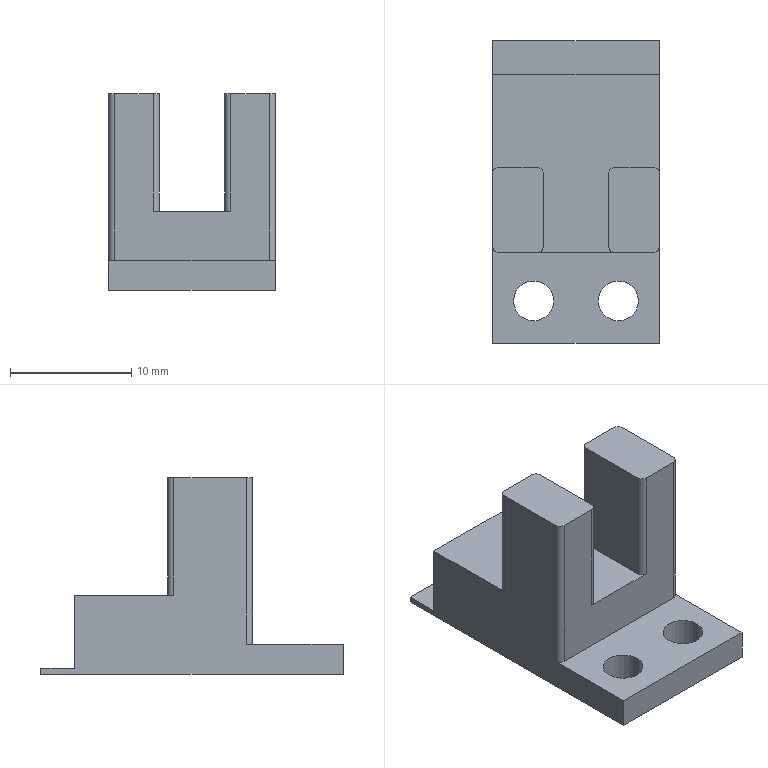Part | NX | features BREP 1 | 1 solid | 28 faces | box 13.8 x 25 x 16.25 mm | volume 2130 mm3 | plane 16 | cylinder 12 | commonest cylinder face diameters 1 x8 3.3 x4
STEP:
#1=CARTESIAN_POINT('',(-3.2,7.5,16.25));
#2=VERTEX_POINT('',#1);
#3=CARTESIAN_POINT('',(-2.7,8.,16.25));
#4=VERTEX_POINT('',#3);
#5=CARTESIAN_POINT('',(-3.2,8.,16.25));
#6=DIRECTION('',(0.,0.,1.));
#7=DIRECTION('',(-1.,0.,0.));
#8=AXIS2_PLACEMENT_3D('',#5,#6,#7);
#9=CIRCLE('',#8,0.5);
#10=EDGE_CURVE('',#2,#4,#9,.T.);
#11=ORIENTED_EDGE('',*,*,#10,.F.);
#12=CARTESIAN_POINT('',(-3.2,7.5,6.55));
#13=VERTEX_POINT('',#12);
#14=CARTESIAN_POINT('',(-3.2,7.5,6.55));
#15=DIRECTION('',(0.,0.,1.));
#16=VECTOR('',#15,1000.);
#17=LINE('',#14,#16);
#18=EDGE_CURVE('',#13,#2,#17,.T.);
#19=ORIENTED_EDGE('',*,*,#18,.F.);
#20=CARTESIAN_POINT('',(-2.7,8.,6.55));
#21=VERTEX_POINT('',#20);
#22=CARTESIAN_POINT('',(-3.2,8.,6.55));
#23=DIRECTION('',(0.,0.,-1.));
#24=DIRECTION('',(-1.,0.,0.));
#25=AXIS2_PLACEMENT_3D('',#22,#23,#24);
#26=CIRCLE('',#25,0.5);
#27=EDGE_CURVE('',#21,#13,#26,.T.);
#28=ORIENTED_EDGE('',*,*,#27,.F.);
#29=CARTESIAN_POINT('',(-2.7,8.,16.25));
#30=DIRECTION('',(0.,0.,-1.));
#31=VECTOR('',#30,1000.);
#32=LINE('',#29,#31);
#33=EDGE_CURVE('',#4,#21,#32,.T.);
#34=ORIENTED_EDGE('',*,*,#33,.F.);
#35=EDGE_LOOP('',(#11,#19,#28,#34));
#36=FACE_BOUND('',#35,.T.);
#37=CARTESIAN_POINT('',(-3.2,8.,16.25));
#38=DIRECTION('',(0.,0.,-1.));
#39=DIRECTION('',(-1.,0.,0.));
#40=AXIS2_PLACEMENT_3D('',#37,#38,#39);
#41=CYLINDRICAL_SURFACE('',#40,0.5);
#42=ADVANCED_FACE('',(#36),#41,.T.);
#43=CARTESIAN_POINT('',(2.7,8.,16.25));
#44=VERTEX_POINT('',#43);
#45=CARTESIAN_POINT('',(3.2,7.5,16.25));
#46=VERTEX_POINT('',#45);
#47=CARTESIAN_POINT('',(3.2,8.,16.25));
#48=DIRECTION('',(0.,0.,1.));
#49=DIRECTION('',(1.,0.,0.));
#50=AXIS2_PLACEMENT_3D('',#47,#48,#49);
#51=CIRCLE('',#50,0.5);
#52=EDGE_CURVE('',#44,#46,#51,.T.);
#53=ORIENTED_EDGE('',*,*,#52,.F.);
#54=CARTESIAN_POINT('',(2.7,8.,6.55));
#55=VERTEX_POINT('',#54);
#56=CARTESIAN_POINT('',(2.7,8.,16.25));
#57=DIRECTION('',(0.,0.,1.));
#58=VECTOR('',#57,1000.);
#59=LINE('',#56,#58);
#60=EDGE_CURVE('',#55,#44,#59,.T.);
#61=ORIENTED_EDGE('',*,*,#60,.F.);
#62=CARTESIAN_POINT('',(3.2,7.5,6.55));
#63=VERTEX_POINT('',#62);
#64=CARTESIAN_POINT('',(3.2,8.,6.55));
#65=DIRECTION('',(0.,0.,-1.));
#66=DIRECTION('',(-1.,0.,0.));
#67=AXIS2_PLACEMENT_3D('',#64,#65,#66);
#68=CIRCLE('',#67,0.5);
#69=EDGE_CURVE('',#63,#55,#68,.T.);
#70=ORIENTED_EDGE('',*,*,#69,.F.);
#71=CARTESIAN_POINT('',(3.2,7.5,6.55));
#72=DIRECTION('',(0.,0.,-1.));
#73=VECTOR('',#72,1000.);
#74=LINE('',#71,#73);
#75=EDGE_CURVE('',#46,#63,#74,.T.);
#76=ORIENTED_EDGE('',*,*,#75,.F.);
#77=EDGE_LOOP('',(#53,#61,#70,#76));
#78=FACE_BOUND('',#77,.T.);
#79=CARTESIAN_POINT('',(3.2,8.,6.55));
#80=DIRECTION('',(0.,0.,-1.));
#81=DIRECTION('',(-1.,0.,0.));
#82=AXIS2_PLACEMENT_3D('',#79,#80,#81);
#83=CYLINDRICAL_SURFACE('',#82,0.5);
#84=ADVANCED_FACE('',(#78),#83,.T.);
#85=CARTESIAN_POINT('',(3.2,14.5,16.25));
#86=VERTEX_POINT('',#85);
#87=CARTESIAN_POINT('',(2.7,14.,16.25));
#88=VERTEX_POINT('',#87);
#89=CARTESIAN_POINT('',(3.2,14.,16.25));
#90=DIRECTION('',(0.,0.,1.));
#91=DIRECTION('',(1.,0.,0.));
#92=AXIS2_PLACEMENT_3D('',#89,#90,#91);
#93=CIRCLE('',#92,0.5);
#94=EDGE_CURVE('',#86,#88,#93,.T.);
#95=ORIENTED_EDGE('',*,*,#94,.F.);
#96=CARTESIAN_POINT('',(3.2,14.5,6.55));
#97=VERTEX_POINT('',#96);
#98=CARTESIAN_POINT('',(3.2,14.5,16.25));
#99=DIRECTION('',(0.,0.,1.));
#100=VECTOR('',#99,1000.);
#101=LINE('',#98,#100);
#102=EDGE_CURVE('',#97,#86,#101,.T.);
#103=ORIENTED_EDGE('',*,*,#102,.F.);
#104=CARTESIAN_POINT('',(2.7,14.,6.55));
#105=VERTEX_POINT('',#104);
#106=CARTESIAN_POINT('',(3.2,14.,6.55));
#107=DIRECTION('',(0.,0.,-1.));
#108=DIRECTION('',(-1.,0.,0.));
#109=AXIS2_PLACEMENT_3D('',#106,#107,#108);
#110=CIRCLE('',#109,0.5);
#111=EDGE_CURVE('',#105,#97,#110,.T.);
#112=ORIENTED_EDGE('',*,*,#111,.F.);
#113=CARTESIAN_POINT('',(2.7,14.,16.25));
#114=DIRECTION('',(0.,0.,-1.));
#115=VECTOR('',#114,1000.);
#116=LINE('',#113,#115);
#117=EDGE_CURVE('',#88,#105,#116,.T.);
#118=ORIENTED_EDGE('',*,*,#117,.F.);
#119=EDGE_LOOP('',(#95,#103,#112,#118));
#120=FACE_BOUND('',#119,.T.);
#121=CARTESIAN_POINT('',(3.2,14.,16.25));
#122=DIRECTION('',(0.,0.,-1.));
#123=DIRECTION('',(-1.,0.,0.));
#124=AXIS2_PLACEMENT_3D('',#121,#122,#123);
#125=CYLINDRICAL_SURFACE('',#124,0.5);
#126=ADVANCED_FACE('',(#120),#125,.T.);
#127=CARTESIAN_POINT('',(-2.7,14.,16.25));
#128=VERTEX_POINT('',#127);
#129=CARTESIAN_POINT('',(-3.2,14.5,16.25));
#130=VERTEX_POINT('',#129);
#131=CARTESIAN_POINT('',(-3.2,14.,16.25));
#132=DIRECTION('',(0.,0.,1.));
#133=DIRECTION('',(-1.,0.,0.));
#134=AXIS2_PLACEMENT_3D('',#131,#132,#133);
#135=CIRCLE('',#134,0.5);
#136=EDGE_CURVE('',#128,#130,#135,.T.);
#137=ORIENTED_EDGE('',*,*,#136,.F.);
#138=CARTESIAN_POINT('',(-2.7,14.,6.55));
#139=VERTEX_POINT('',#138);
#140=CARTESIAN_POINT('',(-2.7,14.,16.25));
#141=DIRECTION('',(0.,0.,1.));
#142=VECTOR('',#141,1000.);
#143=LINE('',#140,#142);
#144=EDGE_CURVE('',#139,#128,#143,.T.);
#145=ORIENTED_EDGE('',*,*,#144,.F.);
#146=CARTESIAN_POINT('',(-3.2,14.5,6.55));
#147=VERTEX_POINT('',#146);
#148=CARTESIAN_POINT('',(-3.2,14.,6.55));
#149=DIRECTION('',(0.,0.,-1.));
#150=DIRECTION('',(-1.,0.,0.));
#151=AXIS2_PLACEMENT_3D('',#148,#149,#150);
#152=CIRCLE('',#151,0.5);
#153=EDGE_CURVE('',#147,#139,#152,.T.);
#154=ORIENTED_EDGE('',*,*,#153,.F.);
#155=CARTESIAN_POINT('',(-3.2,14.5,16.25));
#156=DIRECTION('',(0.,0.,-1.));
#157=VECTOR('',#156,1000.);
#158=LINE('',#155,#157);
#159=EDGE_CURVE('',#130,#147,#158,.T.);
#160=ORIENTED_EDGE('',*,*,#159,.F.);
#161=EDGE_LOOP('',(#137,#145,#154,#160));
#162=FACE_BOUND('',#161,.T.);
#163=CARTESIAN_POINT('',(-3.2,14.,16.25));
#164=DIRECTION('',(0.,0.,-1.));
#165=DIRECTION('',(-1.,0.,0.));
#166=AXIS2_PLACEMENT_3D('',#163,#164,#165);
#167=CYLINDRICAL_SURFACE('',#166,0.5);
#168=ADVANCED_FACE('',(#162),#167,.T.);
#169=CARTESIAN_POINT('',(-6.4,14.5,16.25));
#170=VERTEX_POINT('',#169);
#171=CARTESIAN_POINT('',(-6.9,14.,16.25));
#172=VERTEX_POINT('',#171);
#173=CARTESIAN_POINT('',(-6.4,14.,16.25));
#174=DIRECTION('',(0.,0.,1.));
#175=DIRECTION('',(-1.,0.,0.));
#176=AXIS2_PLACEMENT_3D('',#173,#174,#175);
#177=CIRCLE('',#176,0.5);
#178=EDGE_CURVE('',#170,#172,#177,.T.);
#179=ORIENTED_EDGE('',*,*,#178,.F.);
#180=CARTESIAN_POINT('',(-6.4,14.5,6.55));
#181=VERTEX_POINT('',#180);
#182=CARTESIAN_POINT('',(-6.4,14.5,16.25));
#183=DIRECTION('',(0.,0.,1.));
#184=VECTOR('',#183,1000.);
#185=LINE('',#182,#184);
#186=EDGE_CURVE('',#181,#170,#185,.T.);
#187=ORIENTED_EDGE('',*,*,#186,.F.);
#188=CARTESIAN_POINT('',(-6.9,14.,6.55));
#189=VERTEX_POINT('',#188);
#190=CARTESIAN_POINT('',(-6.4,14.,6.55));
#191=DIRECTION('',(0.,0.,-1.));
#192=DIRECTION('',(-1.,0.,0.));
#193=AXIS2_PLACEMENT_3D('',#190,#191,#192);
#194=CIRCLE('',#193,0.5);
#195=EDGE_CURVE('',#189,#181,#194,.T.);
#196=ORIENTED_EDGE('',*,*,#195,.F.);
#197=CARTESIAN_POINT('',(-6.9,14.,2.5));
#198=DIRECTION('',(0.,0.,-1.));
#199=VECTOR('',#198,1000.);
#200=LINE('',#197,#199);
#201=EDGE_CURVE('',#172,#189,#200,.T.);
#202=ORIENTED_EDGE('',*,*,#201,.F.);
#203=EDGE_LOOP('',(#179,#187,#196,#202));
#204=FACE_BOUND('',#203,.T.);
#205=CARTESIAN_POINT('',(-6.4,14.,2.5));
#206=DIRECTION('',(0.,0.,-1.));
#207=DIRECTION('',(-1.,0.,0.));
#208=AXIS2_PLACEMENT_3D('',#205,#206,#207);
#209=CYLINDRICAL_SURFACE('',#208,0.5);
#210=ADVANCED_FACE('',(#204),#209,.T.);
#211=CARTESIAN_POINT('',(-6.9,8.,16.25));
#212=VERTEX_POINT('',#211);
#213=CARTESIAN_POINT('',(-6.4,7.5,16.25));
#214=VERTEX_POINT('',#213);
#215=CARTESIAN_POINT('',(-6.4,8.,16.25));
#216=DIRECTION('',(0.,0.,1.));
#217=DIRECTION('',(-1.,0.,0.));
#218=AXIS2_PLACEMENT_3D('',#215,#216,#217);
#219=CIRCLE('',#218,0.5);
#220=EDGE_CURVE('',#212,#214,#219,.T.);
#221=ORIENTED_EDGE('',*,*,#220,.F.);
#222=CARTESIAN_POINT('',(-6.9,8.,2.5));
#223=VERTEX_POINT('',#222);
#224=CARTESIAN_POINT('',(-6.9,8.,2.5));
#225=DIRECTION('',(0.,0.,1.));
#226=VECTOR('',#225,1000.);
#227=LINE('',#224,#226);
#228=EDGE_CURVE('',#223,#212,#227,.T.);
#229=ORIENTED_EDGE('',*,*,#228,.F.);
#230=CARTESIAN_POINT('',(-6.4,7.5,2.5));
#231=VERTEX_POINT('',#230);
#232=CARTESIAN_POINT('',(-6.4,8.,2.5));
#233=DIRECTION('',(0.,0.,-1.));
#234=DIRECTION('',(1.,0.,0.));
#235=AXIS2_PLACEMENT_3D('',#232,#233,#234);
#236=CIRCLE('',#235,0.5);
#237=EDGE_CURVE('',#231,#223,#236,.T.);
#238=ORIENTED_EDGE('',*,*,#237,.F.);
#239=CARTESIAN_POINT('',(-6.4,7.5,6.55));
#240=DIRECTION('',(0.,0.,-1.));
#241=VECTOR('',#240,1000.);
#242=LINE('',#239,#241);
#243=EDGE_CURVE('',#214,#231,#242,.T.);
#244=ORIENTED_EDGE('',*,*,#243,.F.);
#245=EDGE_LOOP('',(#221,#229,#238,#244));
#246=FACE_BOUND('',#245,.T.);
#247=CARTESIAN_POINT('',(-6.4,8.,6.55));
#248=DIRECTION('',(0.,0.,-1.));
#249=DIRECTION('',(-1.,0.,0.));
#250=AXIS2_PLACEMENT_3D('',#247,#248,#249);
#251=CYLINDRICAL_SURFACE('',#250,0.5);
#252=ADVANCED_FACE('',(#246),#251,.T.);
#253=CARTESIAN_POINT('',(6.4,7.5,16.25));
#254=VERTEX_POINT('',#253);
#255=CARTESIAN_POINT('',(6.9,8.,16.25));
#256=VERTEX_POINT('',#255);
#257=CARTESIAN_POINT('',(6.4,8.,16.25));
#258=DIRECTION('',(0.,0.,1.));
#259=DIRECTION('',(1.,0.,0.));
#260=AXIS2_PLACEMENT_3D('',#257,#258,#259);
#261=CIRCLE('',#260,0.5);
#262=EDGE_CURVE('',#254,#256,#261,.T.);
#263=ORIENTED_EDGE('',*,*,#262,.F.);
#264=CARTESIAN_POINT('',(6.4,7.5,2.5));
#265=VERTEX_POINT('',#264);
#266=CARTESIAN_POINT('',(6.4,7.5,6.55));
#267=DIRECTION('',(0.,0.,1.));
#268=VECTOR('',#267,1000.);
#269=LINE('',#266,#268);
#270=EDGE_CURVE('',#265,#254,#269,.T.);
#271=ORIENTED_EDGE('',*,*,#270,.F.);
#272=CARTESIAN_POINT('',(6.9,8.,2.5));
#273=VERTEX_POINT('',#272);
#274=CARTESIAN_POINT('',(6.4,8.,2.5));
#275=DIRECTION('',(0.,0.,-1.));
#276=DIRECTION('',(1.,0.,0.));
#277=AXIS2_PLACEMENT_3D('',#274,#275,#276);
#278=CIRCLE('',#277,0.5);
#279=EDGE_CURVE('',#273,#265,#278,.T.);
#280=ORIENTED_EDGE('',*,*,#279,.F.);
#281=CARTESIAN_POINT('',(6.9,8.,2.5));
#282=DIRECTION('',(0.,0.,-1.));
#283=VECTOR('',#282,1000.);
#284=LINE('',#281,#283);
#285=EDGE_CURVE('',#256,#273,#284,.T.);
#286=ORIENTED_EDGE('',*,*,#285,.F.);
#287=EDGE_LOOP('',(#263,#271,#280,#286));
#288=FACE_BOUND('',#287,.T.);
#289=CARTESIAN_POINT('',(6.4,8.,2.5));
#290=DIRECTION('',(0.,0.,-1.));
#291=DIRECTION('',(-1.,0.,0.));
#292=AXIS2_PLACEMENT_3D('',#289,#290,#291);
#293=CYLINDRICAL_SURFACE('',#292,0.5);
#294=ADVANCED_FACE('',(#288),#293,.T.);
#295=CARTESIAN_POINT('',(6.9,14.,16.25));
#296=VERTEX_POINT('',#295);
#297=CARTESIAN_POINT('',(6.4,14.5,16.25));
#298=VERTEX_POINT('',#297);
#299=CARTESIAN_POINT('',(6.4,14.,16.25));
#300=DIRECTION('',(0.,0.,1.));
#301=DIRECTION('',(1.,0.,0.));
#302=AXIS2_PLACEMENT_3D('',#299,#300,#301);
#303=CIRCLE('',#302,0.5);
#304=EDGE_CURVE('',#296,#298,#303,.T.);
#305=ORIENTED_EDGE('',*,*,#304,.F.);
#306=CARTESIAN_POINT('',(6.9,14.,6.55));
#307=VERTEX_POINT('',#306);
#308=CARTESIAN_POINT('',(6.9,14.,2.5));
#309=DIRECTION('',(0.,0.,1.));
#310=VECTOR('',#309,1000.);
#311=LINE('',#308,#310);
#312=EDGE_CURVE('',#307,#296,#311,.T.);
#313=ORIENTED_EDGE('',*,*,#312,.F.);
#314=CARTESIAN_POINT('',(6.4,14.5,6.55));
#315=VERTEX_POINT('',#314);
#316=CARTESIAN_POINT('',(6.4,14.,6.55));
#317=DIRECTION('',(0.,0.,-1.));
#318=DIRECTION('',(-1.,0.,0.));
#319=AXIS2_PLACEMENT_3D('',#316,#317,#318);
#320=CIRCLE('',#319,0.5);
#321=EDGE_CURVE('',#315,#307,#320,.T.);
#322=ORIENTED_EDGE('',*,*,#321,.F.);
#323=CARTESIAN_POINT('',(6.4,14.5,16.25));
#324=DIRECTION('',(0.,0.,-1.));
#325=VECTOR('',#324,1000.);
#326=LINE('',#323,#325);
#327=EDGE_CURVE('',#298,#315,#326,.T.);
#328=ORIENTED_EDGE('',*,*,#327,.F.);
#329=EDGE_LOOP('',(#305,#313,#322,#328));
#330=FACE_BOUND('',#329,.T.);
#331=CARTESIAN_POINT('',(6.4,14.,16.25));
#332=DIRECTION('',(0.,0.,-1.));
#333=DIRECTION('',(-1.,0.,0.));
#334=AXIS2_PLACEMENT_3D('',#331,#332,#333);
#335=CYLINDRICAL_SURFACE('',#334,0.5);
#336=ADVANCED_FACE('',(#330),#335,.T.);
#337=CARTESIAN_POINT('',(-6.9,25.,0.5));
#338=VERTEX_POINT('',#337);
#339=CARTESIAN_POINT('',(-6.9,22.2,0.5));
#340=VERTEX_POINT('',#339);
#341=CARTESIAN_POINT('',(-6.9,22.2,0.5));
#342=DIRECTION('',(0.,-1.,0.));
#343=VECTOR('',#342,1000.);
#344=LINE('',#341,#343);
#345=EDGE_CURVE('',#338,#340,#344,.T.);
#346=ORIENTED_EDGE('',*,*,#345,.T.);
#347=CARTESIAN_POINT('',(6.9,22.2,0.5));
#348=VERTEX_POINT('',#347);
#349=CARTESIAN_POINT('',(-6.9,22.2,0.5));
#350=DIRECTION('',(1.,0.,0.));
#351=VECTOR('',#350,1000.);
#352=LINE('',#349,#351);
#353=EDGE_CURVE('',#340,#348,#352,.T.);
#354=ORIENTED_EDGE('',*,*,#353,.T.);
#355=CARTESIAN_POINT('',(6.9,25.,0.5));
#356=VERTEX_POINT('',#355);
#357=CARTESIAN_POINT('',(6.9,22.2,0.5));
#358=DIRECTION('',(0.,1.,0.));
#359=VECTOR('',#358,1000.);
#360=LINE('',#357,#359);
#361=EDGE_CURVE('',#348,#356,#360,.T.);
#362=ORIENTED_EDGE('',*,*,#361,.T.);
#363=CARTESIAN_POINT('',(-6.9,25.,0.5));
#364=DIRECTION('',(-1.,0.,0.));
#365=VECTOR('',#364,1000.);
#366=LINE('',#363,#365);
#367=EDGE_CURVE('',#356,#338,#366,.T.);
#368=ORIENTED_EDGE('',*,*,#367,.T.);
#369=EDGE_LOOP('',(#346,#354,#362,#368));
#370=FACE_BOUND('',#369,.T.);
#371=CARTESIAN_POINT('',(-6.9,25.,0.5));
#372=DIRECTION('',(0.,0.,-1.));
#373=DIRECTION('',(-1.,0.,0.));
#374=AXIS2_PLACEMENT_3D('',#371,#372,#373);
#375=PLANE('',#374);
#376=ADVANCED_FACE('',(#370),#375,.F.);
#377=CARTESIAN_POINT('',(1.85,3.5,2.5));
#378=VERTEX_POINT('',#377);
#379=CARTESIAN_POINT('',(1.85,3.5,0.));
#380=VERTEX_POINT('',#379);
#381=CARTESIAN_POINT('',(1.85,3.5,-7.2));
#382=DIRECTION('',(0.,0.,1.));
#383=VECTOR('',#382,1000.);
#384=LINE('',#381,#383);
#385=EDGE_CURVE('',#378,#380,#384,.F.);
#386=ORIENTED_EDGE('',*,*,#385,.T.);
#387=CARTESIAN_POINT('',(5.15,3.5,0.));
#388=VERTEX_POINT('',#387);
#389=CARTESIAN_POINT('',(3.5,3.5,0.));
#390=DIRECTION('',(0.,0.,1.));
#391=DIRECTION('',(1.,0.,0.));
#392=AXIS2_PLACEMENT_3D('',#389,#390,#391);
#393=CIRCLE('',#392,1.65);
#394=EDGE_CURVE('',#388,#380,#393,.T.);
#395=ORIENTED_EDGE('',*,*,#394,.F.);
#396=CARTESIAN_POINT('',(5.15,3.5,2.5));
#397=VERTEX_POINT('',#396);
#398=CARTESIAN_POINT('',(5.15,3.5,-7.2));
#399=DIRECTION('',(0.,0.,1.));
#400=VECTOR('',#399,1000.);
#401=LINE('',#398,#400);
#402=EDGE_CURVE('',#397,#388,#401,.F.);
#403=ORIENTED_EDGE('',*,*,#402,.F.);
#404=CARTESIAN_POINT('',(3.5,3.5,2.5));
#405=DIRECTION('',(0.,0.,1.));
#406=DIRECTION('',(1.,0.,0.));
#407=AXIS2_PLACEMENT_3D('',#404,#405,#406);
#408=CIRCLE('',#407,1.65);
#409=EDGE_CURVE('',#397,#378,#408,.T.);
#410=ORIENTED_EDGE('',*,*,#409,.T.);
#411=EDGE_LOOP('',(#386,#395,#403,#410));
#412=FACE_BOUND('',#411,.T.);
#413=CARTESIAN_POINT('',(3.5,3.5,-7.2));
#414=DIRECTION('',(0.,0.,1.));
#415=DIRECTION('',(1.,0.,0.));
#416=AXIS2_PLACEMENT_3D('',#413,#414,#415);
#417=CYLINDRICAL_SURFACE('',#416,1.65);
#418=ADVANCED_FACE('',(#412),#417,.F.);
#419=CARTESIAN_POINT('',(-5.15,3.5,2.5));
#420=VERTEX_POINT('',#419);
#421=CARTESIAN_POINT('',(-5.15,3.5,0.));
#422=VERTEX_POINT('',#421);
#423=CARTESIAN_POINT('',(-5.15,3.5,-7.2));
#424=DIRECTION('',(0.,0.,1.));
#425=VECTOR('',#424,1000.);
#426=LINE('',#423,#425);
#427=EDGE_CURVE('',#420,#422,#426,.F.);
#428=ORIENTED_EDGE('',*,*,#427,.T.);
#429=CARTESIAN_POINT('',(-1.85,3.5,0.));
#430=VERTEX_POINT('',#429);
#431=CARTESIAN_POINT('',(-3.5,3.5,0.));
#432=DIRECTION('',(0.,0.,1.));
#433=DIRECTION('',(1.,0.,0.));
#434=AXIS2_PLACEMENT_3D('',#431,#432,#433);
#435=CIRCLE('',#434,1.65);
#436=EDGE_CURVE('',#430,#422,#435,.T.);
#437=ORIENTED_EDGE('',*,*,#436,.F.);
#438=CARTESIAN_POINT('',(-1.85,3.5,2.5));
#439=VERTEX_POINT('',#438);
#440=CARTESIAN_POINT('',(-1.85,3.5,-7.2));
#441=DIRECTION('',(0.,0.,1.));
#442=VECTOR('',#441,1000.);
#443=LINE('',#440,#442);
#444=EDGE_CURVE('',#439,#430,#443,.F.);
#445=ORIENTED_EDGE('',*,*,#444,.F.);
#446=CARTESIAN_POINT('',(-3.5,3.5,2.5));
#447=DIRECTION('',(0.,0.,1.));
#448=DIRECTION('',(1.,0.,0.));
#449=AXIS2_PLACEMENT_3D('',#446,#447,#448);
#450=CIRCLE('',#449,1.65);
#451=EDGE_CURVE('',#439,#420,#450,.T.);
#452=ORIENTED_EDGE('',*,*,#451,.T.);
#453=EDGE_LOOP('',(#428,#437,#445,#452));
#454=FACE_BOUND('',#453,.T.);
#455=CARTESIAN_POINT('',(-3.5,3.5,-7.2));
#456=DIRECTION('',(0.,0.,1.));
#457=DIRECTION('',(1.,0.,0.));
#458=AXIS2_PLACEMENT_3D('',#455,#456,#457);
#459=CYLINDRICAL_SURFACE('',#458,1.65);
#460=ADVANCED_FACE('',(#454),#459,.F.);
#461=CARTESIAN_POINT('',(6.9,7.5,16.25));
#462=DIRECTION('',(0.,1.,0.));
#463=VECTOR('',#462,1000.);
#464=LINE('',#461,#463);
#465=EDGE_CURVE('',#256,#296,#464,.T.);
#466=ORIENTED_EDGE('',*,*,#465,.T.);
#467=ORIENTED_EDGE('',*,*,#304,.T.);
#468=CARTESIAN_POINT('',(6.9,14.5,16.25));
#469=DIRECTION('',(-1.,0.,0.));
#470=VECTOR('',#469,1000.);
#471=LINE('',#468,#470);
#472=EDGE_CURVE('',#298,#86,#471,.T.);
#473=ORIENTED_EDGE('',*,*,#472,.T.);
#474=ORIENTED_EDGE('',*,*,#94,.T.);
#475=CARTESIAN_POINT('',(2.7,7.5,16.25));
#476=DIRECTION('',(0.,-1.,0.));
#477=VECTOR('',#476,1000.);
#478=LINE('',#475,#477);
#479=EDGE_CURVE('',#88,#44,#478,.T.);
#480=ORIENTED_EDGE('',*,*,#479,.T.);
#481=ORIENTED_EDGE('',*,*,#52,.T.);
#482=CARTESIAN_POINT('',(6.9,7.5,16.25));
#483=DIRECTION('',(1.,0.,0.));
#484=VECTOR('',#483,1000.);
#485=LINE('',#482,#484);
#486=EDGE_CURVE('',#46,#254,#485,.T.);
#487=ORIENTED_EDGE('',*,*,#486,.T.);
#488=ORIENTED_EDGE('',*,*,#262,.T.);
#489=EDGE_LOOP('',(#466,#467,#473,#474,#480,#481,#487,#488));
#490=FACE_BOUND('',#489,.T.);
#491=CARTESIAN_POINT('',(6.9,14.5,16.25));
#492=DIRECTION('',(0.,0.,1.));
#493=DIRECTION('',(1.,0.,0.));
#494=AXIS2_PLACEMENT_3D('',#491,#492,#493);
#495=PLANE('',#494);
#496=ADVANCED_FACE('',(#490),#495,.T.);
#497=ORIENTED_EDGE('',*,*,#479,.F.);
#498=ORIENTED_EDGE('',*,*,#117,.T.);
#499=CARTESIAN_POINT('',(2.7,7.5,6.55));
#500=DIRECTION('',(0.,-1.,0.));
#501=VECTOR('',#500,1000.);
#502=LINE('',#499,#501);
#503=EDGE_CURVE('',#105,#55,#502,.T.);
#504=ORIENTED_EDGE('',*,*,#503,.T.);
#505=ORIENTED_EDGE('',*,*,#60,.T.);
#506=EDGE_LOOP('',(#497,#498,#504,#505));
#507=FACE_BOUND('',#506,.T.);
#508=CARTESIAN_POINT('',(2.7,7.5,16.25));
#509=DIRECTION('',(1.,0.,0.));
#510=DIRECTION('',(0.,0.,-1.));
#511=AXIS2_PLACEMENT_3D('',#508,#509,#510);
#512=PLANE('',#511);
#513=ADVANCED_FACE('',(#507),#512,.F.);
#514=ORIENTED_EDGE('',*,*,#472,.F.);
#515=ORIENTED_EDGE('',*,*,#327,.T.);
#516=CARTESIAN_POINT('',(6.9,14.5,6.55));
#517=DIRECTION('',(-1.,0.,0.));
#518=VECTOR('',#517,1000.);
#519=LINE('',#516,#518);
#520=EDGE_CURVE('',#315,#97,#519,.T.);
#521=ORIENTED_EDGE('',*,*,#520,.T.);
#522=ORIENTED_EDGE('',*,*,#102,.T.);
#523=EDGE_LOOP('',(#514,#515,#521,#522));
#524=FACE_BOUND('',#523,.T.);
#525=CARTESIAN_POINT('',(6.9,14.5,16.25));
#526=DIRECTION('',(0.,-1.,0.));
#527=DIRECTION('',(0.,0.,-1.));
#528=AXIS2_PLACEMENT_3D('',#525,#526,#527);
#529=PLANE('',#528);
#530=ADVANCED_FACE('',(#524),#529,.F.);
#531=CARTESIAN_POINT('',(-6.9,7.5,16.25));
#532=DIRECTION('',(0.,-1.,0.));
#533=VECTOR('',#532,1000.);
#534=LINE('',#531,#533);
#535=EDGE_CURVE('',#172,#212,#534,.T.);
#536=ORIENTED_EDGE('',*,*,#535,.T.);
#537=ORIENTED_EDGE('',*,*,#220,.T.);
#538=CARTESIAN_POINT('',(-6.9,7.5,16.25));
#539=DIRECTION('',(1.,0.,0.));
#540=VECTOR('',#539,1000.);
#541=LINE('',#538,#540);
#542=EDGE_CURVE('',#214,#2,#541,.T.);
#543=ORIENTED_EDGE('',*,*,#542,.T.);
#544=ORIENTED_EDGE('',*,*,#10,.T.);
#545=CARTESIAN_POINT('',(-2.7,7.5,16.25));
#546=DIRECTION('',(0.,1.,0.));
#547=VECTOR('',#546,1000.);
#548=LINE('',#545,#547);
#549=EDGE_CURVE('',#4,#128,#548,.T.);
#550=ORIENTED_EDGE('',*,*,#549,.T.);
#551=ORIENTED_EDGE('',*,*,#136,.T.);
#552=CARTESIAN_POINT('',(-6.9,14.5,16.25));
#553=DIRECTION('',(-1.,0.,0.));
#554=VECTOR('',#553,1000.);
#555=LINE('',#552,#554);
#556=EDGE_CURVE('',#130,#170,#555,.T.);
#557=ORIENTED_EDGE('',*,*,#556,.T.);
#558=ORIENTED_EDGE('',*,*,#178,.T.);
#559=EDGE_LOOP('',(#536,#537,#543,#544,#550,#551,#557,#558));
#560=FACE_BOUND('',#559,.T.);
#561=CARTESIAN_POINT('',(-6.9,14.5,16.25));
#562=DIRECTION('',(0.,0.,-1.));
#563=DIRECTION('',(-1.,0.,0.));
#564=AXIS2_PLACEMENT_3D('',#561,#562,#563);
#565=PLANE('',#564);
#566=ADVANCED_FACE('',(#560),#565,.F.);
#567=CARTESIAN_POINT('',(-6.9,14.5,6.55));
#568=DIRECTION('',(-1.,0.,0.));
#569=VECTOR('',#568,1000.);
#570=LINE('',#567,#569);
#571=EDGE_CURVE('',#147,#181,#570,.T.);
#572=ORIENTED_EDGE('',*,*,#571,.T.);
#573=ORIENTED_EDGE('',*,*,#186,.T.);
#574=ORIENTED_EDGE('',*,*,#556,.F.);
#575=ORIENTED_EDGE('',*,*,#159,.T.);
#576=EDGE_LOOP('',(#572,#573,#574,#575));
#577=FACE_BOUND('',#576,.T.);
#578=CARTESIAN_POINT('',(-6.9,14.5,16.25));
#579=DIRECTION('',(0.,-1.,0.));
#580=DIRECTION('',(0.,0.,-1.));
#581=AXIS2_PLACEMENT_3D('',#578,#579,#580);
#582=PLANE('',#581);
#583=ADVANCED_FACE('',(#577),#582,.F.);
#584=CARTESIAN_POINT('',(-2.7,7.5,6.55));
#585=DIRECTION('',(0.,1.,0.));
#586=VECTOR('',#585,1000.);
#587=LINE('',#584,#586);
#588=EDGE_CURVE('',#21,#139,#587,.T.);
#589=ORIENTED_EDGE('',*,*,#588,.T.);
#590=ORIENTED_EDGE('',*,*,#144,.T.);
#591=ORIENTED_EDGE('',*,*,#549,.F.);
#592=ORIENTED_EDGE('',*,*,#33,.T.);
#593=EDGE_LOOP('',(#589,#590,#591,#592));
#594=FACE_BOUND('',#593,.T.);
#595=CARTESIAN_POINT('',(-2.7,7.5,16.25));
#596=DIRECTION('',(-1.,0.,0.));
#597=DIRECTION('',(0.,0.,1.));
#598=AXIS2_PLACEMENT_3D('',#595,#596,#597);
#599=PLANE('',#598);
#600=ADVANCED_FACE('',(#594),#599,.F.);
#601=CARTESIAN_POINT('',(6.9,22.2,6.55));
#602=VERTEX_POINT('',#601);
#603=CARTESIAN_POINT('',(6.9,22.2,6.55));
#604=DIRECTION('',(0.,0.,-1.));
#605=VECTOR('',#604,1000.);
#606=LINE('',#603,#605);
#607=EDGE_CURVE('',#602,#348,#606,.T.);
#608=ORIENTED_EDGE('',*,*,#607,.T.);
#609=ORIENTED_EDGE('',*,*,#353,.F.);
#610=CARTESIAN_POINT('',(-6.9,22.2,6.55));
#611=VERTEX_POINT('',#610);
#612=CARTESIAN_POINT('',(-6.9,22.2,6.55));
#613=DIRECTION('',(0.,0.,-1.));
#614=VECTOR('',#613,1000.);
#615=LINE('',#612,#614);
#616=EDGE_CURVE('',#611,#340,#615,.T.);
#617=ORIENTED_EDGE('',*,*,#616,.F.);
#618=CARTESIAN_POINT('',(-6.9,22.2,6.55));
#619=DIRECTION('',(-1.,0.,0.));
#620=VECTOR('',#619,1000.);
#621=LINE('',#618,#620);
#622=EDGE_CURVE('',#602,#611,#621,.T.);
#623=ORIENTED_EDGE('',*,*,#622,.F.);
#624=EDGE_LOOP('',(#608,#609,#617,#623));
#625=FACE_BOUND('',#624,.T.);
#626=CARTESIAN_POINT('',(-6.9,22.2,6.55));
#627=DIRECTION('',(0.,-1.,0.));
#628=DIRECTION('',(0.,0.,-1.));
#629=AXIS2_PLACEMENT_3D('',#626,#627,#628);
#630=PLANE('',#629);
#631=ADVANCED_FACE('',(#625),#630,.F.);
#632=CARTESIAN_POINT('',(-6.9,7.5,2.5));
#633=DIRECTION('',(1.,0.,0.));
#634=VECTOR('',#633,1000.);
#635=LINE('',#632,#634);
#636=EDGE_CURVE('',#231,#265,#635,.T.);
#637=ORIENTED_EDGE('',*,*,#636,.T.);
#638=ORIENTED_EDGE('',*,*,#270,.T.);
#639=ORIENTED_EDGE('',*,*,#486,.F.);
#640=ORIENTED_EDGE('',*,*,#75,.T.);
#641=CARTESIAN_POINT('',(-6.9,7.5,6.55));
#642=DIRECTION('',(1.,0.,0.));
#643=VECTOR('',#642,1000.);
#644=LINE('',#641,#643);
#645=EDGE_CURVE('',#13,#63,#644,.T.);
#646=ORIENTED_EDGE('',*,*,#645,.F.);
#647=ORIENTED_EDGE('',*,*,#18,.T.);
#648=ORIENTED_EDGE('',*,*,#542,.F.);
#649=ORIENTED_EDGE('',*,*,#243,.T.);
#650=EDGE_LOOP('',(#637,#638,#639,#640,#646,#647,#648,#649));
#651=FACE_BOUND('',#650,.T.);
#652=CARTESIAN_POINT('',(-6.9,7.5,6.55));
#653=DIRECTION('',(0.,1.,0.));
#654=DIRECTION('',(0.,0.,1.));
#655=AXIS2_PLACEMENT_3D('',#652,#653,#654);
#656=PLANE('',#655);
#657=ADVANCED_FACE('',(#651),#656,.F.);
#658=CARTESIAN_POINT('',(-6.9,25.,0.));
#659=VERTEX_POINT('',#658);
#660=CARTESIAN_POINT('',(-6.9,0.,0.));
#661=VERTEX_POINT('',#660);
#662=CARTESIAN_POINT('',(-6.9,25.,0.));
#663=DIRECTION('',(0.,-1.,0.));
#664=VECTOR('',#663,1000.);
#665=LINE('',#662,#664);
#666=EDGE_CURVE('',#659,#661,#665,.T.);
#667=ORIENTED_EDGE('',*,*,#666,.F.);
#668=CARTESIAN_POINT('',(6.9,25.,0.));
#669=VERTEX_POINT('',#668);
#670=CARTESIAN_POINT('',(6.9,25.,0.));
#671=DIRECTION('',(-1.,0.,0.));
#672=VECTOR('',#671,1000.);
#673=LINE('',#670,#672);
#674=EDGE_CURVE('',#669,#659,#673,.T.);
#675=ORIENTED_EDGE('',*,*,#674,.F.);
#676=CARTESIAN_POINT('',(6.9,0.,0.));
#677=VERTEX_POINT('',#676);
#678=CARTESIAN_POINT('',(6.9,0.,0.));
#679=DIRECTION('',(0.,1.,0.));
#680=VECTOR('',#679,1000.);
#681=LINE('',#678,#680);
#682=EDGE_CURVE('',#677,#669,#681,.T.);
#683=ORIENTED_EDGE('',*,*,#682,.F.);
#684=CARTESIAN_POINT('',(-6.9,0.,0.));
#685=DIRECTION('',(1.,0.,0.));
#686=VECTOR('',#685,1000.);
#687=LINE('',#684,#686);
#688=EDGE_CURVE('',#661,#677,#687,.T.);
#689=ORIENTED_EDGE('',*,*,#688,.F.);
#690=EDGE_LOOP('',(#667,#675,#683,#689));
#691=FACE_BOUND('',#690,.T.);
#692=ORIENTED_EDGE('',*,*,#436,.T.);
#693=CARTESIAN_POINT('',(-3.5,3.5,0.));
#694=DIRECTION('',(0.,0.,1.));
#695=DIRECTION('',(1.,0.,0.));
#696=AXIS2_PLACEMENT_3D('',#693,#694,#695);
#697=CIRCLE('',#696,1.65);
#698=EDGE_CURVE('',#422,#430,#697,.T.);
#699=ORIENTED_EDGE('',*,*,#698,.T.);
#700=EDGE_LOOP('',(#692,#699));
#701=FACE_BOUND('',#700,.T.);
#702=ORIENTED_EDGE('',*,*,#394,.T.);
#703=CARTESIAN_POINT('',(3.5,3.5,0.));
#704=DIRECTION('',(0.,0.,1.));
#705=DIRECTION('',(1.,0.,0.));
#706=AXIS2_PLACEMENT_3D('',#703,#704,#705);
#707=CIRCLE('',#706,1.65);
#708=EDGE_CURVE('',#380,#388,#707,.T.);
#709=ORIENTED_EDGE('',*,*,#708,.T.);
#710=EDGE_LOOP('',(#702,#709));
#711=FACE_BOUND('',#710,.T.);
#712=CARTESIAN_POINT('',(-6.9,0.,0.));
#713=DIRECTION('',(0.,0.,1.));
#714=DIRECTION('',(1.,0.,0.));
#715=AXIS2_PLACEMENT_3D('',#712,#713,#714);
#716=PLANE('',#715);
#717=ADVANCED_FACE('',(#691,#701,#711),#716,.F.);
#718=ORIENTED_EDGE('',*,*,#636,.F.);
#719=ORIENTED_EDGE('',*,*,#237,.T.);
#720=CARTESIAN_POINT('',(-6.9,0.,2.5));
#721=VERTEX_POINT('',#720);
#722=CARTESIAN_POINT('',(-6.9,25.,2.5));
#723=DIRECTION('',(0.,-1.,0.));
#724=VECTOR('',#723,1000.);
#725=LINE('',#722,#724);
#726=EDGE_CURVE('',#223,#721,#725,.T.);
#727=ORIENTED_EDGE('',*,*,#726,.T.);
#728=CARTESIAN_POINT('',(6.9,0.,2.5));
#729=VERTEX_POINT('',#728);
#730=CARTESIAN_POINT('',(-6.9,0.,2.5));
#731=DIRECTION('',(1.,0.,0.));
#732=VECTOR('',#731,1000.);
#733=LINE('',#730,#732);
#734=EDGE_CURVE('',#721,#729,#733,.T.);
#735=ORIENTED_EDGE('',*,*,#734,.T.);
#736=CARTESIAN_POINT('',(6.9,0.,2.5));
#737=DIRECTION('',(0.,1.,0.));
#738=VECTOR('',#737,1000.);
#739=LINE('',#736,#738);
#740=EDGE_CURVE('',#729,#273,#739,.T.);
#741=ORIENTED_EDGE('',*,*,#740,.T.);
#742=ORIENTED_EDGE('',*,*,#279,.T.);
#743=EDGE_LOOP('',(#718,#719,#727,#735,#741,#742));
#744=FACE_BOUND('',#743,.T.);
#745=ORIENTED_EDGE('',*,*,#451,.F.);
#746=CARTESIAN_POINT('',(-3.5,3.5,2.5));
#747=DIRECTION('',(0.,0.,1.));
#748=DIRECTION('',(1.,0.,0.));
#749=AXIS2_PLACEMENT_3D('',#746,#747,#748);
#750=CIRCLE('',#749,1.65);
#751=EDGE_CURVE('',#420,#439,#750,.T.);
#752=ORIENTED_EDGE('',*,*,#751,.F.);
#753=EDGE_LOOP('',(#745,#752));
#754=FACE_BOUND('',#753,.T.);
#755=ORIENTED_EDGE('',*,*,#409,.F.);
#756=CARTESIAN_POINT('',(3.5,3.5,2.5));
#757=DIRECTION('',(0.,0.,1.));
#758=DIRECTION('',(1.,0.,0.));
#759=AXIS2_PLACEMENT_3D('',#756,#757,#758);
#760=CIRCLE('',#759,1.65);
#761=EDGE_CURVE('',#378,#397,#760,.T.);
#762=ORIENTED_EDGE('',*,*,#761,.F.);
#763=EDGE_LOOP('',(#755,#762));
#764=FACE_BOUND('',#763,.T.);
#765=CARTESIAN_POINT('',(-6.9,0.,2.5));
#766=DIRECTION('',(0.,0.,1.));
#767=DIRECTION('',(1.,0.,0.));
#768=AXIS2_PLACEMENT_3D('',#765,#766,#767);
#769=PLANE('',#768);
#770=ADVANCED_FACE('',(#744,#754,#764),#769,.T.);
#771=CARTESIAN_POINT('',(-6.9,25.,2.5));
#772=DIRECTION('',(0.,0.,-1.));
#773=VECTOR('',#772,1000.);
#774=LINE('',#771,#773);
#775=EDGE_CURVE('',#338,#659,#774,.T.);
#776=ORIENTED_EDGE('',*,*,#775,.F.);
#777=ORIENTED_EDGE('',*,*,#367,.F.);
#778=CARTESIAN_POINT('',(6.9,25.,2.5));
#779=DIRECTION('',(0.,0.,-1.));
#780=VECTOR('',#779,1000.);
#781=LINE('',#778,#780);
#782=EDGE_CURVE('',#356,#669,#781,.T.);
#783=ORIENTED_EDGE('',*,*,#782,.T.);
#784=ORIENTED_EDGE('',*,*,#674,.T.);
#785=EDGE_LOOP('',(#776,#777,#783,#784));
#786=FACE_BOUND('',#785,.T.);
#787=CARTESIAN_POINT('',(6.9,25.,2.5));
#788=DIRECTION('',(0.,-1.,0.));
#789=DIRECTION('',(0.,0.,-1.));
#790=AXIS2_PLACEMENT_3D('',#787,#788,#789);
#791=PLANE('',#790);
#792=ADVANCED_FACE('',(#786),#791,.F.);
#793=CARTESIAN_POINT('',(6.9,7.5,6.55));
#794=DIRECTION('',(0.,1.,0.));
#795=VECTOR('',#794,1000.);
#796=LINE('',#793,#795);
#797=EDGE_CURVE('',#307,#602,#796,.T.);
#798=ORIENTED_EDGE('',*,*,#797,.F.);
#799=ORIENTED_EDGE('',*,*,#312,.T.);
#800=ORIENTED_EDGE('',*,*,#465,.F.);
#801=ORIENTED_EDGE('',*,*,#285,.T.);
#802=ORIENTED_EDGE('',*,*,#740,.F.);
#803=CARTESIAN_POINT('',(6.9,0.,2.5));
#804=DIRECTION('',(0.,0.,-1.));
#805=VECTOR('',#804,1000.);
#806=LINE('',#803,#805);
#807=EDGE_CURVE('',#729,#677,#806,.T.);
#808=ORIENTED_EDGE('',*,*,#807,.T.);
#809=ORIENTED_EDGE('',*,*,#682,.T.);
#810=ORIENTED_EDGE('',*,*,#782,.F.);
#811=ORIENTED_EDGE('',*,*,#361,.F.);
#812=ORIENTED_EDGE('',*,*,#607,.F.);
#813=EDGE_LOOP('',(#798,#799,#800,#801,#802,#808,#809,#810,#811,#812));
#814=FACE_BOUND('',#813,.T.);
#815=CARTESIAN_POINT('',(6.9,0.,2.5));
#816=DIRECTION('',(-1.,0.,0.));
#817=DIRECTION('',(0.,-1.,0.));
#818=AXIS2_PLACEMENT_3D('',#815,#816,#817);
#819=PLANE('',#818);
#820=ADVANCED_FACE('',(#814),#819,.F.);
#821=ORIENTED_EDGE('',*,*,#688,.T.);
#822=ORIENTED_EDGE('',*,*,#807,.F.);
#823=ORIENTED_EDGE('',*,*,#734,.F.);
#824=CARTESIAN_POINT('',(-6.9,0.,2.5));
#825=DIRECTION('',(0.,0.,-1.));
#826=VECTOR('',#825,1000.);
#827=LINE('',#824,#826);
#828=EDGE_CURVE('',#721,#661,#827,.T.);
#829=ORIENTED_EDGE('',*,*,#828,.T.);
#830=EDGE_LOOP('',(#821,#822,#823,#829));
#831=FACE_BOUND('',#830,.T.);
#832=CARTESIAN_POINT('',(-6.9,0.,2.5));
#833=DIRECTION('',(0.,1.,0.));
#834=DIRECTION('',(0.,0.,1.));
#835=AXIS2_PLACEMENT_3D('',#832,#833,#834);
#836=PLANE('',#835);
#837=ADVANCED_FACE('',(#831),#836,.F.);
#838=ORIENTED_EDGE('',*,*,#726,.F.);
#839=ORIENTED_EDGE('',*,*,#228,.T.);
#840=ORIENTED_EDGE('',*,*,#535,.F.);
#841=ORIENTED_EDGE('',*,*,#201,.T.);
#842=CARTESIAN_POINT('',(-6.9,7.5,6.55));
#843=DIRECTION('',(0.,-1.,0.));
#844=VECTOR('',#843,1000.);
#845=LINE('',#842,#844);
#846=EDGE_CURVE('',#611,#189,#845,.T.);
#847=ORIENTED_EDGE('',*,*,#846,.F.);
#848=ORIENTED_EDGE('',*,*,#616,.T.);
#849=ORIENTED_EDGE('',*,*,#345,.F.);
#850=ORIENTED_EDGE('',*,*,#775,.T.);
#851=ORIENTED_EDGE('',*,*,#666,.T.);
#852=ORIENTED_EDGE('',*,*,#828,.F.);
#853=EDGE_LOOP('',(#838,#839,#840,#841,#847,#848,#849,#850,#851,#852));
#854=FACE_BOUND('',#853,.T.);
#855=CARTESIAN_POINT('',(-6.9,25.,2.5));
#856=DIRECTION('',(1.,0.,0.));
#857=DIRECTION('',(0.,1.,0.));
#858=AXIS2_PLACEMENT_3D('',#855,#856,#857);
#859=PLANE('',#858);
#860=ADVANCED_FACE('',(#854),#859,.F.);
#861=ORIENTED_EDGE('',*,*,#520,.F.);
#862=ORIENTED_EDGE('',*,*,#321,.T.);
#863=ORIENTED_EDGE('',*,*,#797,.T.);
#864=ORIENTED_EDGE('',*,*,#622,.T.);
#865=ORIENTED_EDGE('',*,*,#846,.T.);
#866=ORIENTED_EDGE('',*,*,#195,.T.);
#867=ORIENTED_EDGE('',*,*,#571,.F.);
#868=ORIENTED_EDGE('',*,*,#153,.T.);
#869=ORIENTED_EDGE('',*,*,#588,.F.);
#870=ORIENTED_EDGE('',*,*,#27,.T.);
#871=ORIENTED_EDGE('',*,*,#645,.T.);
#872=ORIENTED_EDGE('',*,*,#69,.T.);
#873=ORIENTED_EDGE('',*,*,#503,.F.);
#874=ORIENTED_EDGE('',*,*,#111,.T.);
#875=EDGE_LOOP('',(#861,#862,#863,#864,#865,#866,#867,#868,#869,#870,#871,#872,#873,#874));
#876=FACE_BOUND('',#875,.T.);
#877=CARTESIAN_POINT('',(-6.9,22.2,6.55));
#878=DIRECTION('',(0.,0.,-1.));
#879=DIRECTION('',(-1.,0.,0.));
#880=AXIS2_PLACEMENT_3D('',#877,#878,#879);
#881=PLANE('',#880);
#882=ADVANCED_FACE('',(#876),#881,.F.);
#883=ORIENTED_EDGE('',*,*,#698,.F.);
#884=ORIENTED_EDGE('',*,*,#427,.F.);
#885=ORIENTED_EDGE('',*,*,#751,.T.);
#886=ORIENTED_EDGE('',*,*,#444,.T.);
#887=EDGE_LOOP('',(#883,#884,#885,#886));
#888=FACE_BOUND('',#887,.T.);
#889=CARTESIAN_POINT('',(-3.5,3.5,-7.2));
#890=DIRECTION('',(0.,0.,1.));
#891=DIRECTION('',(1.,0.,0.));
#892=AXIS2_PLACEMENT_3D('',#889,#890,#891);
#893=CYLINDRICAL_SURFACE('',#892,1.65);
#894=ADVANCED_FACE('',(#888),#893,.F.);
#895=ORIENTED_EDGE('',*,*,#708,.F.);
#896=ORIENTED_EDGE('',*,*,#385,.F.);
#897=ORIENTED_EDGE('',*,*,#761,.T.);
#898=ORIENTED_EDGE('',*,*,#402,.T.);
#899=EDGE_LOOP('',(#895,#896,#897,#898));
#900=FACE_BOUND('',#899,.T.);
#901=CARTESIAN_POINT('',(3.5,3.5,-7.2));
#902=DIRECTION('',(0.,0.,1.));
#903=DIRECTION('',(1.,0.,0.));
#904=AXIS2_PLACEMENT_3D('',#901,#902,#903);
#905=CYLINDRICAL_SURFACE('',#904,1.65);
#906=ADVANCED_FACE('',(#900),#905,.F.);
#907=CLOSED_SHELL('',(#42,#84,#126,#168,#210,#252,#294,#336,#376,#418,#460,#496,#513,#530,#566,#583,#600,#631,#657,#717,#770,#792,#820,#837,#860,#882,#894,#906));
#908=MANIFOLD_SOLID_BREP('',#907);
#909=(LENGTH_UNIT()NAMED_UNIT(*)SI_UNIT(.MILLI.,.METRE.));
#910=UNCERTAINTY_MEASURE_WITH_UNIT(LENGTH_MEASURE(0.00001),#909,'','');
#911=(NAMED_UNIT(*)PLANE_ANGLE_UNIT()SI_UNIT($,.RADIAN.));
#912=(NAMED_UNIT(*)SI_UNIT($,.STERADIAN.)SOLID_ANGLE_UNIT());
#913=(GEOMETRIC_REPRESENTATION_CONTEXT(3)GLOBAL_UNCERTAINTY_ASSIGNED_CONTEXT((#910))GLOBAL_UNIT_ASSIGNED_CONTEXT((#909,#911,#912))REPRESENTATION_CONTEXT('',''));
#914=ADVANCED_BREP_SHAPE_REPRESENTATION('',(#908),#913);